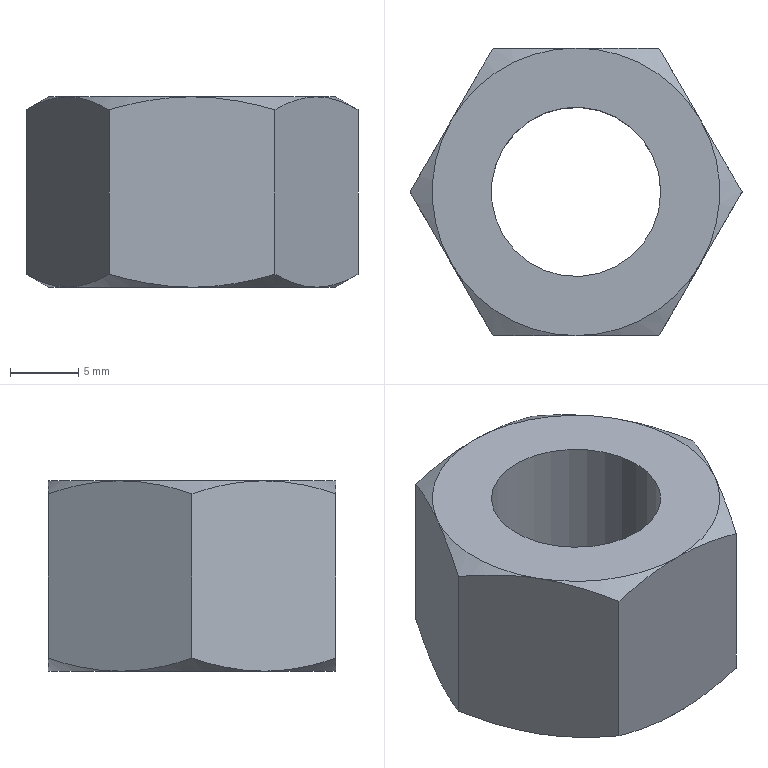Part | NX | 1 solid | 21 faces | box 24.249 x 21 x 13.9 mm | volume 3616 mm3 | cone 12 | plane 8 | cylinder 1 | commonest cylinder face diameters 12.376 x1
STEP:
#1=CARTESIAN_POINT('',(-9.093,5.25,13.9));
#2=VERTEX_POINT('',#1);
#3=CARTESIAN_POINT('',(0.,10.5,13.9));
#4=VERTEX_POINT('',#3);
#5=CARTESIAN_POINT('',(0.,0.,13.9));
#6=DIRECTION('',(0.,0.,-1.));
#7=DIRECTION('',(-1.,0.,0.));
#8=AXIS2_PLACEMENT_3D('',#5,#6,#7);
#9=CIRCLE('',#8,10.5);
#10=EDGE_CURVE('',#2,#4,#9,.T.);
#11=ORIENTED_EDGE('',*,*,#10,.F.);
#12=CARTESIAN_POINT('',(-9.093,-5.25,13.9));
#13=VERTEX_POINT('',#12);
#14=CARTESIAN_POINT('',(0.,0.,13.9));
#15=DIRECTION('',(0.,0.,-1.));
#16=DIRECTION('',(-1.,0.,0.));
#17=AXIS2_PLACEMENT_3D('',#14,#15,#16);
#18=CIRCLE('',#17,10.5);
#19=EDGE_CURVE('',#13,#2,#18,.T.);
#20=ORIENTED_EDGE('',*,*,#19,.F.);
#21=CARTESIAN_POINT('',(0.,-10.5,13.9));
#22=VERTEX_POINT('',#21);
#23=CARTESIAN_POINT('',(0.,0.,13.9));
#24=DIRECTION('',(0.,0.,-1.));
#25=DIRECTION('',(-1.,0.,0.));
#26=AXIS2_PLACEMENT_3D('',#23,#24,#25);
#27=CIRCLE('',#26,10.5);
#28=EDGE_CURVE('',#22,#13,#27,.T.);
#29=ORIENTED_EDGE('',*,*,#28,.F.);
#30=CARTESIAN_POINT('',(9.093,-5.25,13.9));
#31=VERTEX_POINT('',#30);
#32=CARTESIAN_POINT('',(0.,0.,13.9));
#33=DIRECTION('',(0.,0.,-1.));
#34=DIRECTION('',(-1.,0.,0.));
#35=AXIS2_PLACEMENT_3D('',#32,#33,#34);
#36=CIRCLE('',#35,10.5);
#37=EDGE_CURVE('',#31,#22,#36,.T.);
#38=ORIENTED_EDGE('',*,*,#37,.F.);
#39=CARTESIAN_POINT('',(9.093,5.25,13.9));
#40=VERTEX_POINT('',#39);
#41=CARTESIAN_POINT('',(0.,0.,13.9));
#42=DIRECTION('',(0.,0.,-1.));
#43=DIRECTION('',(-1.,0.,0.));
#44=AXIS2_PLACEMENT_3D('',#41,#42,#43);
#45=CIRCLE('',#44,10.5);
#46=EDGE_CURVE('',#40,#31,#45,.T.);
#47=ORIENTED_EDGE('',*,*,#46,.F.);
#48=CARTESIAN_POINT('',(0.,0.,13.9));
#49=DIRECTION('',(0.,0.,-1.));
#50=DIRECTION('',(-1.,0.,0.));
#51=AXIS2_PLACEMENT_3D('',#48,#49,#50);
#52=CIRCLE('',#51,10.5);
#53=EDGE_CURVE('',#4,#40,#52,.T.);
#54=ORIENTED_EDGE('',*,*,#53,.F.);
#55=EDGE_LOOP('',(#11,#20,#29,#38,#47,#54));
#56=FACE_BOUND('',#55,.T.);
#57=CARTESIAN_POINT('',(6.188,0.,13.9));
#58=VERTEX_POINT('',#57);
#59=CARTESIAN_POINT('',(0.,0.,13.9));
#60=DIRECTION('',(0.,0.,-1.));
#61=DIRECTION('',(1.,0.,0.));
#62=AXIS2_PLACEMENT_3D('',#59,#60,#61);
#63=CIRCLE('',#62,6.188);
#64=EDGE_CURVE('',#58,#58,#63,.T.);
#65=ORIENTED_EDGE('',*,*,#64,.T.);
#66=EDGE_LOOP('',(#65));
#67=FACE_BOUND('',#66,.T.);
#68=CARTESIAN_POINT('',(0.,21.,13.9));
#69=DIRECTION('',(0.,0.,1.));
#70=DIRECTION('',(-1.,0.,0.));
#71=AXIS2_PLACEMENT_3D('',#68,#69,#70);
#72=PLANE('',#71);
#73=ADVANCED_FACE('',(#56,#67),#72,.T.);
#74=CARTESIAN_POINT('',(-9.093,-5.25,0.));
#75=VERTEX_POINT('',#74);
#76=CARTESIAN_POINT('',(-9.093,5.25,0.));
#77=VERTEX_POINT('',#76);
#78=CARTESIAN_POINT('',(0.,0.,0.));
#79=DIRECTION('',(0.,0.,-1.));
#80=DIRECTION('',(-1.,0.,0.));
#81=AXIS2_PLACEMENT_3D('',#78,#79,#80);
#82=CIRCLE('',#81,10.5);
#83=EDGE_CURVE('',#75,#77,#82,.T.);
#84=ORIENTED_EDGE('',*,*,#83,.T.);
#85=CARTESIAN_POINT('',(0.,10.5,0.));
#86=VERTEX_POINT('',#85);
#87=CARTESIAN_POINT('',(0.,0.,0.));
#88=DIRECTION('',(0.,0.,-1.));
#89=DIRECTION('',(-1.,0.,0.));
#90=AXIS2_PLACEMENT_3D('',#87,#88,#89);
#91=CIRCLE('',#90,10.5);
#92=EDGE_CURVE('',#77,#86,#91,.T.);
#93=ORIENTED_EDGE('',*,*,#92,.T.);
#94=CARTESIAN_POINT('',(9.093,5.25,0.));
#95=VERTEX_POINT('',#94);
#96=CARTESIAN_POINT('',(0.,0.,0.));
#97=DIRECTION('',(0.,0.,-1.));
#98=DIRECTION('',(-1.,0.,0.));
#99=AXIS2_PLACEMENT_3D('',#96,#97,#98);
#100=CIRCLE('',#99,10.5);
#101=EDGE_CURVE('',#86,#95,#100,.T.);
#102=ORIENTED_EDGE('',*,*,#101,.T.);
#103=CARTESIAN_POINT('',(9.093,-5.25,0.));
#104=VERTEX_POINT('',#103);
#105=CARTESIAN_POINT('',(0.,0.,0.));
#106=DIRECTION('',(0.,0.,-1.));
#107=DIRECTION('',(-1.,0.,0.));
#108=AXIS2_PLACEMENT_3D('',#105,#106,#107);
#109=CIRCLE('',#108,10.5);
#110=EDGE_CURVE('',#95,#104,#109,.T.);
#111=ORIENTED_EDGE('',*,*,#110,.T.);
#112=CARTESIAN_POINT('',(0.,-10.5,0.));
#113=VERTEX_POINT('',#112);
#114=CARTESIAN_POINT('',(0.,0.,0.));
#115=DIRECTION('',(0.,0.,-1.));
#116=DIRECTION('',(-1.,0.,0.));
#117=AXIS2_PLACEMENT_3D('',#114,#115,#116);
#118=CIRCLE('',#117,10.5);
#119=EDGE_CURVE('',#104,#113,#118,.T.);
#120=ORIENTED_EDGE('',*,*,#119,.T.);
#121=CARTESIAN_POINT('',(0.,0.,0.));
#122=DIRECTION('',(0.,0.,-1.));
#123=DIRECTION('',(-1.,0.,0.));
#124=AXIS2_PLACEMENT_3D('',#121,#122,#123);
#125=CIRCLE('',#124,10.5);
#126=EDGE_CURVE('',#113,#75,#125,.T.);
#127=ORIENTED_EDGE('',*,*,#126,.T.);
#128=EDGE_LOOP('',(#84,#93,#102,#111,#120,#127));
#129=FACE_BOUND('',#128,.T.);
#130=CARTESIAN_POINT('',(6.188,0.,0.));
#131=VERTEX_POINT('',#130);
#132=CARTESIAN_POINT('',(0.,0.,0.));
#133=DIRECTION('',(0.,0.,-1.));
#134=DIRECTION('',(1.,0.,0.));
#135=AXIS2_PLACEMENT_3D('',#132,#133,#134);
#136=CIRCLE('',#135,6.188);
#137=EDGE_CURVE('',#131,#131,#136,.T.);
#138=ORIENTED_EDGE('',*,*,#137,.F.);
#139=EDGE_LOOP('',(#138));
#140=FACE_BOUND('',#139,.T.);
#141=CARTESIAN_POINT('',(0.,21.,0.));
#142=DIRECTION('',(0.,0.,1.));
#143=DIRECTION('',(-1.,0.,0.));
#144=AXIS2_PLACEMENT_3D('',#141,#142,#143);
#145=PLANE('',#144);
#146=ADVANCED_FACE('',(#129,#140),#145,.F.);
#147=CARTESIAN_POINT('',(12.124,0.,12.962));
#148=VERTEX_POINT('',#147);
#149=CARTESIAN_POINT('',(12.124,0.,0.9378));
#150=VERTEX_POINT('',#149);
#151=CARTESIAN_POINT('',(12.124,0.,13.9));
#152=DIRECTION('',(0.,0.,-1.));
#153=VECTOR('',#152,1.);
#154=LINE('',#151,#153);
#155=EDGE_CURVE('',#148,#150,#154,.T.);
#156=ORIENTED_EDGE('',*,*,#155,.T.);
#157=CARTESIAN_POINT('',(12.124,0.,0.9378));
#158=CARTESIAN_POINT('',(11.134,1.715,0.3661));
#159=CARTESIAN_POINT('',(10.128,3.458,0.));
#160=CARTESIAN_POINT('',(9.093,5.25,0.));
#161=B_SPLINE_CURVE_WITH_KNOTS('',3,(#157,#158,#159,#160),.UNSPECIFIED.,.F.,.F.,(4,4),(0.,1.),.UNSPECIFIED.);
#162=EDGE_CURVE('',#150,#95,#161,.T.);
#163=ORIENTED_EDGE('',*,*,#162,.T.);
#164=CARTESIAN_POINT('',(6.062,10.5,0.9378));
#165=VERTEX_POINT('',#164);
#166=CARTESIAN_POINT('',(9.093,5.25,0.));
#167=CARTESIAN_POINT('',(8.059,7.042,0.));
#168=CARTESIAN_POINT('',(7.052,8.785,0.3661));
#169=CARTESIAN_POINT('',(6.062,10.5,0.9378));
#170=B_SPLINE_CURVE_WITH_KNOTS('',3,(#166,#167,#168,#169),.UNSPECIFIED.,.F.,.F.,(4,4),(0.,1.),.UNSPECIFIED.);
#171=EDGE_CURVE('',#95,#165,#170,.T.);
#172=ORIENTED_EDGE('',*,*,#171,.T.);
#173=CARTESIAN_POINT('',(6.062,10.5,12.962));
#174=VERTEX_POINT('',#173);
#175=CARTESIAN_POINT('',(6.062,10.5,13.9));
#176=DIRECTION('',(0.,0.,-1.));
#177=VECTOR('',#176,1.);
#178=LINE('',#175,#177);
#179=EDGE_CURVE('',#174,#165,#178,.T.);
#180=ORIENTED_EDGE('',*,*,#179,.F.);
#181=CARTESIAN_POINT('',(6.062,10.5,12.962));
#182=CARTESIAN_POINT('',(7.052,8.785,13.534));
#183=CARTESIAN_POINT('',(8.059,7.042,13.9));
#184=CARTESIAN_POINT('',(9.093,5.25,13.9));
#185=B_SPLINE_CURVE_WITH_KNOTS('',3,(#181,#182,#183,#184),.UNSPECIFIED.,.F.,.F.,(4,4),(0.,1.),.UNSPECIFIED.);
#186=EDGE_CURVE('',#174,#40,#185,.T.);
#187=ORIENTED_EDGE('',*,*,#186,.T.);
#188=CARTESIAN_POINT('',(9.093,5.25,13.9));
#189=CARTESIAN_POINT('',(10.128,3.458,13.9));
#190=CARTESIAN_POINT('',(11.134,1.715,13.534));
#191=CARTESIAN_POINT('',(12.124,0.,12.962));
#192=B_SPLINE_CURVE_WITH_KNOTS('',3,(#188,#189,#190,#191),.UNSPECIFIED.,.F.,.F.,(4,4),(0.,1.),.UNSPECIFIED.);
#193=EDGE_CURVE('',#40,#148,#192,.T.);
#194=ORIENTED_EDGE('',*,*,#193,.T.);
#195=EDGE_LOOP('',(#156,#163,#172,#180,#187,#194));
#196=FACE_OUTER_BOUND('',#195,.T.);
#197=CARTESIAN_POINT('',(6.062,10.5,13.9));
#198=DIRECTION('',(0.866,0.5,0.));
#199=DIRECTION('',(0.5,-0.866,0.));
#200=AXIS2_PLACEMENT_3D('',#197,#198,#199);
#201=PLANE('',#200);
#202=ADVANCED_FACE('',(#196),#201,.T.);
#203=CARTESIAN_POINT('',(6.062,-10.5,12.962));
#204=VERTEX_POINT('',#203);
#205=CARTESIAN_POINT('',(6.062,-10.5,0.9378));
#206=VERTEX_POINT('',#205);
#207=CARTESIAN_POINT('',(6.062,-10.5,13.9));
#208=DIRECTION('',(0.,0.,-1.));
#209=VECTOR('',#208,1.);
#210=LINE('',#207,#209);
#211=EDGE_CURVE('',#204,#206,#210,.T.);
#212=ORIENTED_EDGE('',*,*,#211,.T.);
#213=CARTESIAN_POINT('',(6.062,-10.5,0.9378));
#214=CARTESIAN_POINT('',(7.052,-8.785,0.3661));
#215=CARTESIAN_POINT('',(8.059,-7.042,0.));
#216=CARTESIAN_POINT('',(9.093,-5.25,0.));
#217=B_SPLINE_CURVE_WITH_KNOTS('',3,(#213,#214,#215,#216),.UNSPECIFIED.,.F.,.F.,(4,4),(0.,1.),.UNSPECIFIED.);
#218=EDGE_CURVE('',#206,#104,#217,.T.);
#219=ORIENTED_EDGE('',*,*,#218,.T.);
#220=CARTESIAN_POINT('',(9.093,-5.25,0.));
#221=CARTESIAN_POINT('',(10.128,-3.458,0.));
#222=CARTESIAN_POINT('',(11.134,-1.715,0.3661));
#223=CARTESIAN_POINT('',(12.124,0.,0.9378));
#224=B_SPLINE_CURVE_WITH_KNOTS('',3,(#220,#221,#222,#223),.UNSPECIFIED.,.F.,.F.,(4,4),(0.,1.),.UNSPECIFIED.);
#225=EDGE_CURVE('',#104,#150,#224,.T.);
#226=ORIENTED_EDGE('',*,*,#225,.T.);
#227=ORIENTED_EDGE('',*,*,#155,.F.);
#228=CARTESIAN_POINT('',(12.124,0.,12.962));
#229=CARTESIAN_POINT('',(11.134,-1.715,13.534));
#230=CARTESIAN_POINT('',(10.128,-3.458,13.9));
#231=CARTESIAN_POINT('',(9.093,-5.25,13.9));
#232=B_SPLINE_CURVE_WITH_KNOTS('',3,(#228,#229,#230,#231),.UNSPECIFIED.,.F.,.F.,(4,4),(0.,1.),.UNSPECIFIED.);
#233=EDGE_CURVE('',#148,#31,#232,.T.);
#234=ORIENTED_EDGE('',*,*,#233,.T.);
#235=CARTESIAN_POINT('',(9.093,-5.25,13.9));
#236=CARTESIAN_POINT('',(8.059,-7.042,13.9));
#237=CARTESIAN_POINT('',(7.052,-8.785,13.534));
#238=CARTESIAN_POINT('',(6.062,-10.5,12.962));
#239=B_SPLINE_CURVE_WITH_KNOTS('',3,(#235,#236,#237,#238),.UNSPECIFIED.,.F.,.F.,(4,4),(0.,1.),.UNSPECIFIED.);
#240=EDGE_CURVE('',#31,#204,#239,.T.);
#241=ORIENTED_EDGE('',*,*,#240,.T.);
#242=EDGE_LOOP('',(#212,#219,#226,#227,#234,#241));
#243=FACE_OUTER_BOUND('',#242,.T.);
#244=CARTESIAN_POINT('',(12.124,0.,13.9));
#245=DIRECTION('',(0.866,-0.5,0.));
#246=DIRECTION('',(-0.5,-0.866,0.));
#247=AXIS2_PLACEMENT_3D('',#244,#245,#246);
#248=PLANE('',#247);
#249=ADVANCED_FACE('',(#243),#248,.T.);
#250=CARTESIAN_POINT('',(-6.062,-10.5,12.962));
#251=VERTEX_POINT('',#250);
#252=CARTESIAN_POINT('',(-6.062,-10.5,0.9378));
#253=VERTEX_POINT('',#252);
#254=CARTESIAN_POINT('',(-6.062,-10.5,13.9));
#255=DIRECTION('',(0.,0.,-1.));
#256=VECTOR('',#255,1.);
#257=LINE('',#254,#256);
#258=EDGE_CURVE('',#251,#253,#257,.T.);
#259=ORIENTED_EDGE('',*,*,#258,.T.);
#260=CARTESIAN_POINT('',(-6.062,-10.5,0.9378));
#261=CARTESIAN_POINT('',(-4.082,-10.5,0.3661));
#262=CARTESIAN_POINT('',(-2.069,-10.5,0.));
#263=CARTESIAN_POINT('',(0.,-10.5,0.));
#264=B_SPLINE_CURVE_WITH_KNOTS('',3,(#260,#261,#262,#263),.UNSPECIFIED.,.F.,.F.,(4,4),(0.,1.),.UNSPECIFIED.);
#265=EDGE_CURVE('',#253,#113,#264,.T.);
#266=ORIENTED_EDGE('',*,*,#265,.T.);
#267=CARTESIAN_POINT('',(0.,-10.5,0.));
#268=CARTESIAN_POINT('',(2.069,-10.5,0.));
#269=CARTESIAN_POINT('',(4.082,-10.5,0.3661));
#270=CARTESIAN_POINT('',(6.062,-10.5,0.9378));
#271=B_SPLINE_CURVE_WITH_KNOTS('',3,(#267,#268,#269,#270),.UNSPECIFIED.,.F.,.F.,(4,4),(0.,1.),.UNSPECIFIED.);
#272=EDGE_CURVE('',#113,#206,#271,.T.);
#273=ORIENTED_EDGE('',*,*,#272,.T.);
#274=ORIENTED_EDGE('',*,*,#211,.F.);
#275=CARTESIAN_POINT('',(6.062,-10.5,12.962));
#276=CARTESIAN_POINT('',(4.082,-10.5,13.534));
#277=CARTESIAN_POINT('',(2.069,-10.5,13.9));
#278=CARTESIAN_POINT('',(0.,-10.5,13.9));
#279=B_SPLINE_CURVE_WITH_KNOTS('',3,(#275,#276,#277,#278),.UNSPECIFIED.,.F.,.F.,(4,4),(0.,1.),.UNSPECIFIED.);
#280=EDGE_CURVE('',#204,#22,#279,.T.);
#281=ORIENTED_EDGE('',*,*,#280,.T.);
#282=CARTESIAN_POINT('',(0.,-10.5,13.9));
#283=CARTESIAN_POINT('',(-2.069,-10.5,13.9));
#284=CARTESIAN_POINT('',(-4.082,-10.5,13.534));
#285=CARTESIAN_POINT('',(-6.062,-10.5,12.962));
#286=B_SPLINE_CURVE_WITH_KNOTS('',3,(#282,#283,#284,#285),.UNSPECIFIED.,.F.,.F.,(4,4),(0.,1.),.UNSPECIFIED.);
#287=EDGE_CURVE('',#22,#251,#286,.T.);
#288=ORIENTED_EDGE('',*,*,#287,.T.);
#289=EDGE_LOOP('',(#259,#266,#273,#274,#281,#288));
#290=FACE_OUTER_BOUND('',#289,.T.);
#291=CARTESIAN_POINT('',(6.062,-10.5,13.9));
#292=DIRECTION('',(0.,-1.,0.));
#293=DIRECTION('',(0.,0.,1.));
#294=AXIS2_PLACEMENT_3D('',#291,#292,#293);
#295=PLANE('',#294);
#296=ADVANCED_FACE('',(#290),#295,.T.);
#297=CARTESIAN_POINT('',(-12.124,0.,12.962));
#298=VERTEX_POINT('',#297);
#299=CARTESIAN_POINT('',(-12.124,0.,0.9378));
#300=VERTEX_POINT('',#299);
#301=CARTESIAN_POINT('',(-12.124,0.,13.9));
#302=DIRECTION('',(0.,0.,-1.));
#303=VECTOR('',#302,1.);
#304=LINE('',#301,#303);
#305=EDGE_CURVE('',#298,#300,#304,.T.);
#306=ORIENTED_EDGE('',*,*,#305,.T.);
#307=CARTESIAN_POINT('',(-12.124,0.,0.9378));
#308=CARTESIAN_POINT('',(-11.134,-1.715,0.3661));
#309=CARTESIAN_POINT('',(-10.128,-3.458,0.));
#310=CARTESIAN_POINT('',(-9.093,-5.25,0.));
#311=B_SPLINE_CURVE_WITH_KNOTS('',3,(#307,#308,#309,#310),.UNSPECIFIED.,.F.,.F.,(4,4),(0.,1.),.UNSPECIFIED.);
#312=EDGE_CURVE('',#300,#75,#311,.T.);
#313=ORIENTED_EDGE('',*,*,#312,.T.);
#314=CARTESIAN_POINT('',(-9.093,-5.25,0.));
#315=CARTESIAN_POINT('',(-8.059,-7.042,0.));
#316=CARTESIAN_POINT('',(-7.052,-8.785,0.3661));
#317=CARTESIAN_POINT('',(-6.062,-10.5,0.9378));
#318=B_SPLINE_CURVE_WITH_KNOTS('',3,(#314,#315,#316,#317),.UNSPECIFIED.,.F.,.F.,(4,4),(0.,1.),.UNSPECIFIED.);
#319=EDGE_CURVE('',#75,#253,#318,.T.);
#320=ORIENTED_EDGE('',*,*,#319,.T.);
#321=ORIENTED_EDGE('',*,*,#258,.F.);
#322=CARTESIAN_POINT('',(-6.062,-10.5,12.962));
#323=CARTESIAN_POINT('',(-7.052,-8.785,13.534));
#324=CARTESIAN_POINT('',(-8.059,-7.042,13.9));
#325=CARTESIAN_POINT('',(-9.093,-5.25,13.9));
#326=B_SPLINE_CURVE_WITH_KNOTS('',3,(#322,#323,#324,#325),.UNSPECIFIED.,.F.,.F.,(4,4),(0.,1.),.UNSPECIFIED.);
#327=EDGE_CURVE('',#251,#13,#326,.T.);
#328=ORIENTED_EDGE('',*,*,#327,.T.);
#329=CARTESIAN_POINT('',(-9.093,-5.25,13.9));
#330=CARTESIAN_POINT('',(-10.128,-3.458,13.9));
#331=CARTESIAN_POINT('',(-11.134,-1.715,13.534));
#332=CARTESIAN_POINT('',(-12.124,0.,12.962));
#333=B_SPLINE_CURVE_WITH_KNOTS('',3,(#329,#330,#331,#332),.UNSPECIFIED.,.F.,.F.,(4,4),(0.,1.),.UNSPECIFIED.);
#334=EDGE_CURVE('',#13,#298,#333,.T.);
#335=ORIENTED_EDGE('',*,*,#334,.T.);
#336=EDGE_LOOP('',(#306,#313,#320,#321,#328,#335));
#337=FACE_OUTER_BOUND('',#336,.T.);
#338=CARTESIAN_POINT('',(-6.062,-10.5,13.9));
#339=DIRECTION('',(-0.866,-0.5,0.));
#340=DIRECTION('',(-0.5,0.866,0.));
#341=AXIS2_PLACEMENT_3D('',#338,#339,#340);
#342=PLANE('',#341);
#343=ADVANCED_FACE('',(#337),#342,.T.);
#344=CARTESIAN_POINT('',(-6.062,10.5,12.962));
#345=VERTEX_POINT('',#344);
#346=CARTESIAN_POINT('',(-6.062,10.5,0.9378));
#347=VERTEX_POINT('',#346);
#348=CARTESIAN_POINT('',(-6.062,10.5,13.9));
#349=DIRECTION('',(0.,0.,-1.));
#350=VECTOR('',#349,1.);
#351=LINE('',#348,#350);
#352=EDGE_CURVE('',#345,#347,#351,.T.);
#353=ORIENTED_EDGE('',*,*,#352,.T.);
#354=CARTESIAN_POINT('',(-6.062,10.5,0.9378));
#355=CARTESIAN_POINT('',(-7.052,8.785,0.3661));
#356=CARTESIAN_POINT('',(-8.059,7.042,0.));
#357=CARTESIAN_POINT('',(-9.093,5.25,0.));
#358=B_SPLINE_CURVE_WITH_KNOTS('',3,(#354,#355,#356,#357),.UNSPECIFIED.,.F.,.F.,(4,4),(0.,1.),.UNSPECIFIED.);
#359=EDGE_CURVE('',#347,#77,#358,.T.);
#360=ORIENTED_EDGE('',*,*,#359,.T.);
#361=CARTESIAN_POINT('',(-9.093,5.25,0.));
#362=CARTESIAN_POINT('',(-10.128,3.458,0.));
#363=CARTESIAN_POINT('',(-11.134,1.715,0.3661));
#364=CARTESIAN_POINT('',(-12.124,0.,0.9378));
#365=B_SPLINE_CURVE_WITH_KNOTS('',3,(#361,#362,#363,#364),.UNSPECIFIED.,.F.,.F.,(4,4),(0.,1.),.UNSPECIFIED.);
#366=EDGE_CURVE('',#77,#300,#365,.T.);
#367=ORIENTED_EDGE('',*,*,#366,.T.);
#368=ORIENTED_EDGE('',*,*,#305,.F.);
#369=CARTESIAN_POINT('',(-12.124,0.,12.962));
#370=CARTESIAN_POINT('',(-11.134,1.715,13.534));
#371=CARTESIAN_POINT('',(-10.128,3.458,13.9));
#372=CARTESIAN_POINT('',(-9.093,5.25,13.9));
#373=B_SPLINE_CURVE_WITH_KNOTS('',3,(#369,#370,#371,#372),.UNSPECIFIED.,.F.,.F.,(4,4),(0.,1.),.UNSPECIFIED.);
#374=EDGE_CURVE('',#298,#2,#373,.T.);
#375=ORIENTED_EDGE('',*,*,#374,.T.);
#376=CARTESIAN_POINT('',(-9.093,5.25,13.9));
#377=CARTESIAN_POINT('',(-8.059,7.042,13.9));
#378=CARTESIAN_POINT('',(-7.052,8.785,13.534));
#379=CARTESIAN_POINT('',(-6.062,10.5,12.962));
#380=B_SPLINE_CURVE_WITH_KNOTS('',3,(#376,#377,#378,#379),.UNSPECIFIED.,.F.,.F.,(4,4),(0.,1.),.UNSPECIFIED.);
#381=EDGE_CURVE('',#2,#345,#380,.T.);
#382=ORIENTED_EDGE('',*,*,#381,.T.);
#383=EDGE_LOOP('',(#353,#360,#367,#368,#375,#382));
#384=FACE_OUTER_BOUND('',#383,.T.);
#385=CARTESIAN_POINT('',(-12.124,0.,13.9));
#386=DIRECTION('',(-0.866,0.5,0.));
#387=DIRECTION('',(0.5,0.866,0.));
#388=AXIS2_PLACEMENT_3D('',#385,#386,#387);
#389=PLANE('',#388);
#390=ADVANCED_FACE('',(#384),#389,.T.);
#391=ORIENTED_EDGE('',*,*,#179,.T.);
#392=CARTESIAN_POINT('',(6.062,10.5,0.9378));
#393=CARTESIAN_POINT('',(4.082,10.5,0.3661));
#394=CARTESIAN_POINT('',(2.069,10.5,0.));
#395=CARTESIAN_POINT('',(0.,10.5,0.));
#396=B_SPLINE_CURVE_WITH_KNOTS('',3,(#392,#393,#394,#395),.UNSPECIFIED.,.F.,.F.,(4,4),(0.,1.),.UNSPECIFIED.);
#397=EDGE_CURVE('',#165,#86,#396,.T.);
#398=ORIENTED_EDGE('',*,*,#397,.T.);
#399=CARTESIAN_POINT('',(0.,10.5,0.));
#400=CARTESIAN_POINT('',(-2.069,10.5,0.));
#401=CARTESIAN_POINT('',(-4.082,10.5,0.3661));
#402=CARTESIAN_POINT('',(-6.062,10.5,0.9378));
#403=B_SPLINE_CURVE_WITH_KNOTS('',3,(#399,#400,#401,#402),.UNSPECIFIED.,.F.,.F.,(4,4),(0.,1.),.UNSPECIFIED.);
#404=EDGE_CURVE('',#86,#347,#403,.T.);
#405=ORIENTED_EDGE('',*,*,#404,.T.);
#406=ORIENTED_EDGE('',*,*,#352,.F.);
#407=CARTESIAN_POINT('',(-6.062,10.5,12.962));
#408=CARTESIAN_POINT('',(-4.082,10.5,13.534));
#409=CARTESIAN_POINT('',(-2.069,10.5,13.9));
#410=CARTESIAN_POINT('',(0.,10.5,13.9));
#411=B_SPLINE_CURVE_WITH_KNOTS('',3,(#407,#408,#409,#410),.UNSPECIFIED.,.F.,.F.,(4,4),(0.,1.),.UNSPECIFIED.);
#412=EDGE_CURVE('',#345,#4,#411,.T.);
#413=ORIENTED_EDGE('',*,*,#412,.T.);
#414=CARTESIAN_POINT('',(0.,10.5,13.9));
#415=CARTESIAN_POINT('',(2.069,10.5,13.9));
#416=CARTESIAN_POINT('',(4.082,10.5,13.534));
#417=CARTESIAN_POINT('',(6.062,10.5,12.962));
#418=B_SPLINE_CURVE_WITH_KNOTS('',3,(#414,#415,#416,#417),.UNSPECIFIED.,.F.,.F.,(4,4),(0.,1.),.UNSPECIFIED.);
#419=EDGE_CURVE('',#4,#174,#418,.T.);
#420=ORIENTED_EDGE('',*,*,#419,.T.);
#421=EDGE_LOOP('',(#391,#398,#405,#406,#413,#420));
#422=FACE_OUTER_BOUND('',#421,.T.);
#423=CARTESIAN_POINT('',(-6.062,10.5,13.9));
#424=DIRECTION('',(0.,1.,0.));
#425=DIRECTION('',(0.,0.,-1.));
#426=AXIS2_PLACEMENT_3D('',#423,#424,#425);
#427=PLANE('',#426);
#428=ADVANCED_FACE('',(#422),#427,.T.);
#429=ORIENTED_EDGE('',*,*,#419,.F.);
#430=ORIENTED_EDGE('',*,*,#53,.T.);
#431=ORIENTED_EDGE('',*,*,#186,.F.);
#432=EDGE_LOOP('',(#429,#430,#431));
#433=FACE_OUTER_BOUND('',#432,.T.);
#434=CARTESIAN_POINT('',(0.,0.,12.962));
#435=DIRECTION('',(0.,0.,-1.));
#436=DIRECTION('',(1.,0.,0.));
#437=AXIS2_PLACEMENT_3D('',#434,#435,#436);
#438=CONICAL_SURFACE('',#437,12.124,60.);
#439=ADVANCED_FACE('',(#433),#438,.T.);
#440=ORIENTED_EDGE('',*,*,#10,.T.);
#441=ORIENTED_EDGE('',*,*,#412,.F.);
#442=ORIENTED_EDGE('',*,*,#381,.F.);
#443=EDGE_LOOP('',(#440,#441,#442));
#444=FACE_OUTER_BOUND('',#443,.T.);
#445=CARTESIAN_POINT('',(0.,0.,12.962));
#446=DIRECTION('',(0.,0.,-1.));
#447=DIRECTION('',(1.,0.,0.));
#448=AXIS2_PLACEMENT_3D('',#445,#446,#447);
#449=CONICAL_SURFACE('',#448,12.124,60.);
#450=ADVANCED_FACE('',(#444),#449,.T.);
#451=ORIENTED_EDGE('',*,*,#19,.T.);
#452=ORIENTED_EDGE('',*,*,#374,.F.);
#453=ORIENTED_EDGE('',*,*,#334,.F.);
#454=EDGE_LOOP('',(#451,#452,#453));
#455=FACE_OUTER_BOUND('',#454,.T.);
#456=CARTESIAN_POINT('',(0.,0.,12.962));
#457=DIRECTION('',(0.,0.,-1.));
#458=DIRECTION('',(1.,0.,0.));
#459=AXIS2_PLACEMENT_3D('',#456,#457,#458);
#460=CONICAL_SURFACE('',#459,12.124,60.);
#461=ADVANCED_FACE('',(#455),#460,.T.);
#462=ORIENTED_EDGE('',*,*,#28,.T.);
#463=ORIENTED_EDGE('',*,*,#327,.F.);
#464=ORIENTED_EDGE('',*,*,#287,.F.);
#465=EDGE_LOOP('',(#462,#463,#464));
#466=FACE_OUTER_BOUND('',#465,.T.);
#467=CARTESIAN_POINT('',(0.,0.,12.962));
#468=DIRECTION('',(0.,0.,-1.));
#469=DIRECTION('',(1.,0.,0.));
#470=AXIS2_PLACEMENT_3D('',#467,#468,#469);
#471=CONICAL_SURFACE('',#470,12.124,60.);
#472=ADVANCED_FACE('',(#466),#471,.T.);
#473=ORIENTED_EDGE('',*,*,#37,.T.);
#474=ORIENTED_EDGE('',*,*,#280,.F.);
#475=ORIENTED_EDGE('',*,*,#240,.F.);
#476=EDGE_LOOP('',(#473,#474,#475));
#477=FACE_OUTER_BOUND('',#476,.T.);
#478=CARTESIAN_POINT('',(0.,0.,12.962));
#479=DIRECTION('',(0.,0.,-1.));
#480=DIRECTION('',(1.,0.,0.));
#481=AXIS2_PLACEMENT_3D('',#478,#479,#480);
#482=CONICAL_SURFACE('',#481,12.124,60.);
#483=ADVANCED_FACE('',(#477),#482,.T.);
#484=ORIENTED_EDGE('',*,*,#46,.T.);
#485=ORIENTED_EDGE('',*,*,#233,.F.);
#486=ORIENTED_EDGE('',*,*,#193,.F.);
#487=EDGE_LOOP('',(#484,#485,#486));
#488=FACE_OUTER_BOUND('',#487,.T.);
#489=CARTESIAN_POINT('',(0.,0.,12.962));
#490=DIRECTION('',(0.,0.,-1.));
#491=DIRECTION('',(1.,0.,0.));
#492=AXIS2_PLACEMENT_3D('',#489,#490,#491);
#493=CONICAL_SURFACE('',#492,12.124,60.);
#494=ADVANCED_FACE('',(#488),#493,.T.);
#495=ORIENTED_EDGE('',*,*,#404,.F.);
#496=ORIENTED_EDGE('',*,*,#92,.F.);
#497=ORIENTED_EDGE('',*,*,#359,.F.);
#498=EDGE_LOOP('',(#495,#496,#497));
#499=FACE_OUTER_BOUND('',#498,.T.);
#500=CARTESIAN_POINT('',(0.,0.,0.));
#501=DIRECTION('',(0.,0.,1.));
#502=DIRECTION('',(-1.,0.,0.));
#503=AXIS2_PLACEMENT_3D('',#500,#501,#502);
#504=CONICAL_SURFACE('',#503,10.5,60.);
#505=ADVANCED_FACE('',(#499),#504,.T.);
#506=ORIENTED_EDGE('',*,*,#101,.F.);
#507=ORIENTED_EDGE('',*,*,#397,.F.);
#508=ORIENTED_EDGE('',*,*,#171,.F.);
#509=EDGE_LOOP('',(#506,#507,#508));
#510=FACE_OUTER_BOUND('',#509,.T.);
#511=CARTESIAN_POINT('',(0.,0.,0.));
#512=DIRECTION('',(0.,0.,1.));
#513=DIRECTION('',(-1.,0.,0.));
#514=AXIS2_PLACEMENT_3D('',#511,#512,#513);
#515=CONICAL_SURFACE('',#514,10.5,60.);
#516=ADVANCED_FACE('',(#510),#515,.T.);
#517=ORIENTED_EDGE('',*,*,#366,.F.);
#518=ORIENTED_EDGE('',*,*,#83,.F.);
#519=ORIENTED_EDGE('',*,*,#312,.F.);
#520=EDGE_LOOP('',(#517,#518,#519));
#521=FACE_OUTER_BOUND('',#520,.T.);
#522=CARTESIAN_POINT('',(0.,0.,0.));
#523=DIRECTION('',(0.,0.,1.));
#524=DIRECTION('',(-1.,0.,0.));
#525=AXIS2_PLACEMENT_3D('',#522,#523,#524);
#526=CONICAL_SURFACE('',#525,10.5,60.);
#527=ADVANCED_FACE('',(#521),#526,.T.);
#528=ORIENTED_EDGE('',*,*,#319,.F.);
#529=ORIENTED_EDGE('',*,*,#126,.F.);
#530=ORIENTED_EDGE('',*,*,#265,.F.);
#531=EDGE_LOOP('',(#528,#529,#530));
#532=FACE_OUTER_BOUND('',#531,.T.);
#533=CARTESIAN_POINT('',(0.,0.,0.));
#534=DIRECTION('',(0.,0.,1.));
#535=DIRECTION('',(-1.,0.,0.));
#536=AXIS2_PLACEMENT_3D('',#533,#534,#535);
#537=CONICAL_SURFACE('',#536,10.5,60.);
#538=ADVANCED_FACE('',(#532),#537,.T.);
#539=ORIENTED_EDGE('',*,*,#119,.F.);
#540=ORIENTED_EDGE('',*,*,#218,.F.);
#541=ORIENTED_EDGE('',*,*,#272,.F.);
#542=EDGE_LOOP('',(#539,#540,#541));
#543=FACE_OUTER_BOUND('',#542,.T.);
#544=CARTESIAN_POINT('',(0.,0.,0.));
#545=DIRECTION('',(0.,0.,1.));
#546=DIRECTION('',(-1.,0.,0.));
#547=AXIS2_PLACEMENT_3D('',#544,#545,#546);
#548=CONICAL_SURFACE('',#547,10.5,60.);
#549=ADVANCED_FACE('',(#543),#548,.T.);
#550=ORIENTED_EDGE('',*,*,#110,.F.);
#551=ORIENTED_EDGE('',*,*,#162,.F.);
#552=ORIENTED_EDGE('',*,*,#225,.F.);
#553=EDGE_LOOP('',(#550,#551,#552));
#554=FACE_OUTER_BOUND('',#553,.T.);
#555=CARTESIAN_POINT('',(0.,0.,0.));
#556=DIRECTION('',(0.,0.,1.));
#557=DIRECTION('',(-1.,0.,0.));
#558=AXIS2_PLACEMENT_3D('',#555,#556,#557);
#559=CONICAL_SURFACE('',#558,10.5,60.);
#560=ADVANCED_FACE('',(#554),#559,.T.);
#561=ORIENTED_EDGE('',*,*,#64,.F.);
#562=EDGE_LOOP('',(#561));
#563=FACE_BOUND('',#562,.T.);
#564=ORIENTED_EDGE('',*,*,#137,.T.);
#565=EDGE_LOOP('',(#564));
#566=FACE_BOUND('',#565,.T.);
#567=CARTESIAN_POINT('',(0.,0.,13.9));
#568=DIRECTION('',(0.,0.,-1.));
#569=DIRECTION('',(1.,0.,0.));
#570=AXIS2_PLACEMENT_3D('',#567,#568,#569);
#571=CYLINDRICAL_SURFACE('',#570,6.188);
#572=ADVANCED_FACE('',(#563,#566),#571,.F.);
#573=CLOSED_SHELL('',(#73,#146,#202,#249,#296,#343,#390,#428,#439,#450,#461,#472,#483,#494,#505,#516,#527,#538,#549,#560,#572));
#574=MANIFOLD_SOLID_BREP('',#573);
#575=(LENGTH_UNIT()NAMED_UNIT(*)SI_UNIT(.MILLI.,.METRE.));
#576=UNCERTAINTY_MEASURE_WITH_UNIT(LENGTH_MEASURE(0.0508),#575,'','');
#577=(NAMED_UNIT(*)PLANE_ANGLE_UNIT()SI_UNIT($,.RADIAN.));
#578=PLANE_ANGLE_MEASURE_WITH_UNIT(PLANE_ANGLE_MEASURE(0.01745),#577);
#579=DIMENSIONAL_EXPONENTS(0.,0.,0.,0.,0.,0.,0.);
#580=(CONVERSION_BASED_UNIT('DEGREE',#578)NAMED_UNIT(#579)PLANE_ANGLE_UNIT());
#581=(NAMED_UNIT(*)SI_UNIT($,.STERADIAN.)SOLID_ANGLE_UNIT());
#582=(GEOMETRIC_REPRESENTATION_CONTEXT(3)GLOBAL_UNCERTAINTY_ASSIGNED_CONTEXT((#576))GLOBAL_UNIT_ASSIGNED_CONTEXT((#575,#580,#581))REPRESENTATION_CONTEXT('',''));
#583=ADVANCED_BREP_SHAPE_REPRESENTATION('',(#574),#582);